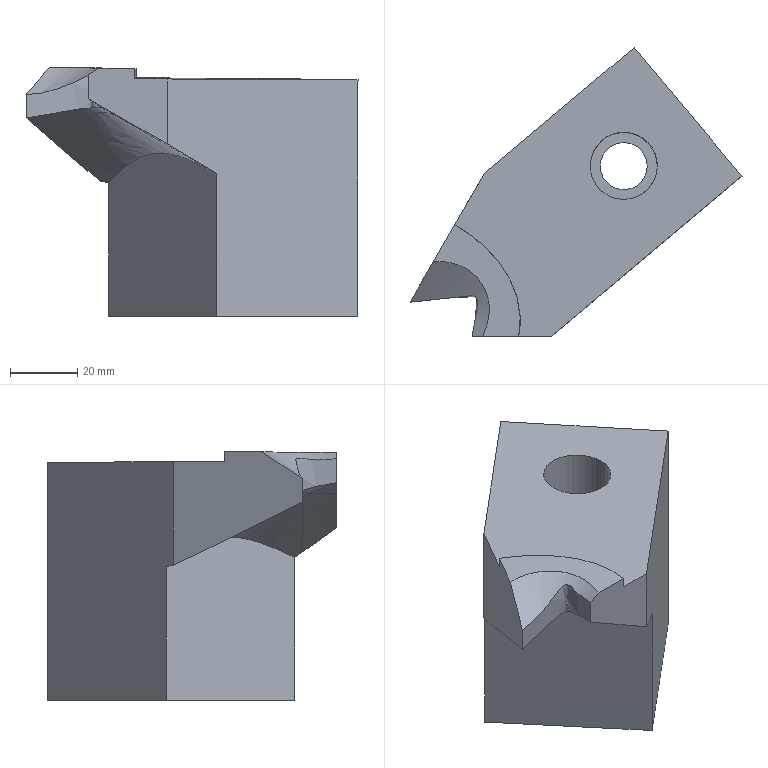Part | NX | features solid 2 | 1 solid | 24 faces | box 98.892 x 86.008 x 74.081 mm | volume 202305 mm3 | spline 14 | plane 8 | cylinder 2 | commonest cylinder face diameters 14 x1 20 x1